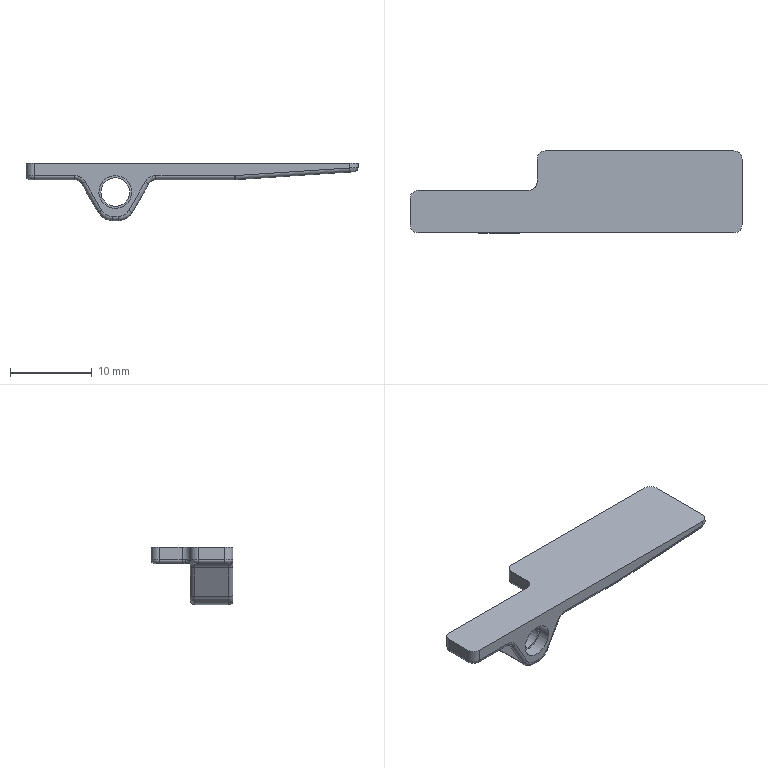NC program | Mastercam | posted with a generic post | part box 40.5 x 10 x 7 mm
Lines 3535 to 4637 of 12178:
(2 BM/BNOS |TOOL - 1|DIA. OFF. - 1|LEN. - 1|TOOL DIA. - 2.)
N7130 T1 M6
N7132 G0 G54 G90 X-19.75 Y.8 C0. B0. S8000 M3
N7134 G43 H1 Z25.
N7136 Z0.
N7138 G1 Z-5. F600.
N7140 Y4. F2000.
N7142 G0 Z0.
N7144 Z25.
N7146 X-19.67 Y4.258
N7148 Z0.
N7150 G1 Z-5. F600.
N7152 Y.538 F2000.
N7154 X-19.668 Y.512
N7156 X-19.662 Y.487
N7158 X-19.653 Y.463
N7160 X-19.642 Y.441
N7162 X-19.63 Y.424
N7164 X-19.619 Y.411
N7166 X-19.608 Y.405
N7168 X-19.599 Y.407
N7170 X-19.593 Y.417
N7172 X-19.591 Y.437
N7174 Y4.362
N7176 X-19.588 Y4.381
N7178 X-19.582 Y4.399
N7180 X-19.573 Y4.415
N7182 X-19.562 Y4.428
N7184 X-19.551 Y4.438
N7186 X-19.539 Y4.444
N7188 X-19.528 Y4.445
N7190 X-19.519 Y4.442
N7192 X-19.513 Y4.432
N7194 X-19.511 Y4.417
N7196 Y.382
N7198 X-19.509 Y.364
N7200 X-19.502 Y.348
N7202 X-19.494 Y.333
N7204 X-19.483 Y.322
N7206 X-19.471 Y.313
N7208 X-19.459 Y.308
N7210 X-19.448 Y.307
N7212 X-19.439 Y.311
N7214 X-19.433 Y.321
N7216 X-19.431 Y.336
N7218 Y4.465
N7220 X-19.429 Y4.481
N7222 X-19.423 Y4.493
N7224 X-19.414 Y4.503
N7226 X-19.403 Y4.51
N7228 X-19.391 Y4.514
N7230 X-19.379
N7232 X-19.369 Y4.511
N7234 X-19.36 Y4.505
N7236 X-19.354 Y4.495
N7238 X-19.351 Y4.481
N7240 Y.318
N7242 X-19.349 Y.303
N7244 X-19.343 Y.29
N7246 X-19.334 Y.28
N7248 X-19.323 Y.273
N7250 X-19.311 Y.268
N7252 X-19.3 Y.267
N7254 X-19.289 Y.27
N7256 X-19.28 Y.276
N7258 X-19.274 Y.286
N7260 X-19.272 Y.3
N7262 Y4.496
N7264 X-19.269 Y4.51
N7266 X-19.263 Y4.522
N7268 X-19.254 Y4.53
N7270 X-19.243 Y4.536
N7272 X-19.232 Y4.538
N7274 X-19.22 Y4.537
N7276 X-19.209 Y4.533
N7278 X-19.2 Y4.525
N7280 X-19.194 Y4.514
N7282 X-19.192 Y4.5
N7284 Y.3
N7286 X-19.19 Y.286
N7288 X-19.183 Y.274
N7290 X-19.175 Y.267
N7292 X-19.164 Y.262
N7294 X-19.152 Y.26
N7296 X-19.14 Y.262
N7298 X-19.129 Y.267
N7300 X-19.12 Y.274
N7302 X-19.114 Y.286
N7304 X-19.112 Y.3
N7306 Y4.5
N7308 X-19.11 Y4.514
N7310 X-19.104 Y4.526
N7312 X-19.095 Y4.533
N7314 X-19.084 Y4.538
N7316 X-19.072 Y4.54
N7318 X-19.06 Y4.538
N7320 X-19.05 Y4.533
N7322 X-19.041 Y4.526
N7324 X-19.035 Y4.514
N7326 X-19.032 Y4.5
N7328 Y.3
N7330 X-19.03 Y.286
N7332 X-19.024 Y.274
N7334 X-19.015 Y.267
N7336 X-19.004 Y.262
N7338 X-18.992 Y.26
N7340 X-18.981 Y.262
N7342 X-18.97 Y.267
N7344 X-18.961 Y.274
N7346 X-18.955 Y.286
N7348 X-18.953 Y.3
N7350 Y4.5
N7352 X-18.95 Y4.514
N7354 X-18.944 Y4.526
N7356 X-18.935 Y4.533
N7358 X-18.924 Y4.538
N7360 X-18.913 Y4.54
N7362 X-18.901 Y4.538
N7364 X-18.89 Y4.533
N7366 X-18.881 Y4.526
N7368 X-18.875 Y4.514
N7370 X-18.873 Y4.5
N7372 Y.3
N7374 X-18.871 Y.286
N7376 X-18.865 Y.274
N7378 X-18.856 Y.267
N7380 X-18.845 Y.262
N7382 X-18.833 Y.26
N7384 X-18.821 Y.262
N7386 X-18.81 Y.267
N7388 X-18.801 Y.274
N7390 X-18.795 Y.286
N7392 X-18.793 Y.3
N7394 Y4.5
N7396 X-18.791 Y4.514
N7398 X-18.785 Y4.526
N7400 X-18.776 Y4.533
N7402 X-18.765 Y4.538
N7404 X-18.753 Y4.54
N7406 X-18.741 Y4.538
N7408 X-18.731 Y4.533
N7410 X-18.722 Y4.526
N7412 X-18.716 Y4.514
N7414 X-18.713 Y4.5
N7416 Y.3
N7418 X-18.711 Y.286
N7420 X-18.705 Y.274
N7422 X-18.696 Y.267
N7424 X-18.685 Y.262
N7426 X-18.673 Y.26
N7428 X-18.662 Y.262
N7430 X-18.651 Y.267
N7432 X-18.642 Y.274
N7434 X-18.636 Y.286
N7436 X-18.634 Y.3
N7438 Y4.5
N7440 X-18.631 Y4.514
N7442 X-18.625 Y4.526
N7444 X-18.616 Y4.533
N7446 X-18.606 Y4.538
N7448 X-18.594 Y4.54
N7450 X-18.582 Y4.538
N7452 X-18.571 Y4.533
N7454 X-18.562 Y4.526
N7456 X-18.556 Y4.514
N7458 X-18.554 Y4.5
N7460 Y.3
N7462 X-18.552 Y.286
N7464 X-18.546 Y.274
N7466 X-18.537 Y.267
N7468 X-18.526 Y.262
N7470 X-18.514 Y.26
N7472 X-18.502 Y.262
N7474 X-18.491 Y.267
N7476 X-18.482 Y.274
N7478 X-18.476 Y.286
N7480 X-18.474 Y.3
N7482 Y4.5
N7484 X-18.472 Y4.514
N7486 X-18.466 Y4.526
N7488 X-18.457 Y4.533
N7490 X-18.446 Y4.538
N7492 X-18.434 Y4.54
N7494 X-18.422 Y4.538
N7496 X-18.412 Y4.533
N7498 X-18.403 Y4.526
N7500 X-18.397 Y4.514
N7502 X-18.394 Y4.5
N7504 Y.3
N7506 X-18.392 Y.286
N7508 X-18.386 Y.274
N7510 X-18.377 Y.267
N7512 X-18.366 Y.262
N7514 X-18.354 Y.26
N7516 X-18.343 Y.262
N7518 X-18.332 Y.267
N7520 X-18.323 Y.274
N7522 X-18.317 Y.286
N7524 X-18.315 Y.3
N7526 Y4.5
N7528 X-18.312 Y4.514
N7530 X-18.306 Y4.526
N7532 X-18.297 Y4.533
N7534 X-18.287 Y4.538
N7536 X-18.275 Y4.54
N7538 X-18.263 Y4.538
N7540 X-18.252 Y4.533
N7542 X-18.243 Y4.526
N7544 X-18.237 Y4.514
N7546 X-18.235 Y4.5
N7548 Y.3
N7550 X-18.233 Y.286
N7552 X-18.227 Y.274
N7554 X-18.218 Y.267
N7556 X-18.207 Y.262
N7558 X-18.195 Y.26
N7560 X-18.183 Y.262
N7562 X-18.172 Y.267
N7564 X-18.163 Y.274
N7566 X-18.157 Y.286
N7568 X-18.155 Y.3
N7570 Y4.5
N7572 X-18.153 Y4.514
N7574 X-18.147 Y4.526
N7576 X-18.138 Y4.533
N7578 X-18.127 Y4.538
N7580 X-18.115 Y4.54
N7582 X-18.103 Y4.538
N7584 X-18.093 Y4.533
N7586 X-18.084 Y4.526
N7588 X-18.078 Y4.514
N7590 X-18.075 Y4.5
N7592 Y.3
N7594 X-18.073 Y.286
N7596 X-18.067 Y.274
N7598 X-18.058 Y.267
N7600 X-18.047 Y.262
N7602 X-18.035 Y.26
N7604 X-18.024 Y.262
N7606 X-18.013 Y.267
N7608 X-18.004 Y.274
N7610 X-17.998 Y.286
N7612 X-17.996 Y.3
N7614 Y4.5
N7616 X-17.993 Y4.514
N7618 X-17.987 Y4.526
N7620 X-17.978 Y4.533
N7622 X-17.968 Y4.538
N7624 X-17.956 Y4.54
N7626 X-17.944 Y4.538
N7628 X-17.933 Y4.533
N7630 X-17.924 Y4.526
N7632 X-17.918 Y4.514
N7634 X-17.916 Y4.5
N7636 Y.3
N7638 X-17.914 Y.286
N7640 X-17.908 Y.274
N7642 X-17.899 Y.267
N7644 X-17.888 Y.262
N7646 X-17.876 Y.26
N7648 X-17.864 Y.262
N7650 X-17.853 Y.267
N7652 X-17.844 Y.274
N7654 X-17.838 Y.286
N7656 X-17.836 Y.3
N7658 Y4.5
N7660 X-17.834 Y4.514
N7662 X-17.828 Y4.526
N7664 X-17.819 Y4.533
N7666 X-17.808 Y4.538
N7668 X-17.796 Y4.54
N7670 X-17.784 Y4.538
N7672 X-17.774 Y4.533
N7674 X-17.765 Y4.526
N7676 X-17.759 Y4.514
N7678 X-17.756 Y4.5
N7680 Y.3
N7682 X-17.754 Y.286
N7684 X-17.748 Y.274
N7686 X-17.739 Y.267
N7688 X-17.728 Y.262
N7690 X-17.717 Y.26
N7692 X-17.705 Y.262
N7694 X-17.694 Y.267
N7696 X-17.685 Y.274
N7698 X-17.679 Y.286
N7700 X-17.677 Y.3
N7702 Y4.5
N7704 X-17.674 Y4.514
N7706 X-17.668 Y4.526
N7708 X-17.659 Y4.533
N7710 X-17.649 Y4.538
N7712 X-17.637 Y4.54
N7714 X-17.625 Y4.538
N7716 X-17.614 Y4.533
N7718 X-17.605 Y4.526
N7720 X-17.599 Y4.514
N7722 X-17.597 Y4.5
N7724 Y.3
N7726 X-17.595 Y.286
N7728 X-17.589 Y.274
N7730 X-17.58 Y.267
N7732 X-17.569 Y.262
N7734 X-17.557 Y.26
N7736 X-17.545 Y.262
N7738 X-17.534 Y.267
N7740 X-17.525 Y.274
N7742 X-17.519 Y.286
N7744 X-17.517 Y.3
N7746 Y4.5
N7748 X-17.515 Y4.514
N7750 X-17.509 Y4.526
N7752 X-17.5 Y4.533
N7754 X-17.489 Y4.538
N7756 X-17.477 Y4.54
N7758 X-17.465 Y4.538
N7760 X-17.455 Y4.533
N7762 X-17.446 Y4.526
N7764 X-17.44 Y4.514
N7766 X-17.437 Y4.5
N7768 Y.3
N7770 X-17.435 Y.286
N7772 X-17.429 Y.274
N7774 X-17.42 Y.267
N7776 X-17.409 Y.262
N7778 X-17.398 Y.26
N7780 X-17.386 Y.262
N7782 X-17.375 Y.267
N7784 X-17.366 Y.274
N7786 X-17.36 Y.286
N7788 X-17.358 Y.3
N7790 Y4.5
N7792 X-17.355 Y4.514
N7794 X-17.349 Y4.526
N7796 X-17.34 Y4.533
N7798 X-17.33 Y4.538
N7800 X-17.318 Y4.54
N7802 X-17.306 Y4.538
N7804 X-17.295 Y4.533
N7806 X-17.286 Y4.526
N7808 X-17.28 Y4.514
N7810 X-17.278 Y4.5
N7812 Y.3
N7814 X-17.276 Y.286
N7816 X-17.27 Y.274
N7818 X-17.261 Y.267
N7820 X-17.25 Y.262
N7822 X-17.238 Y.26
N7824 X-17.226 Y.262
N7826 X-17.215 Y.267
N7828 X-17.206 Y.274
N7830 X-17.2 Y.286
N7832 X-17.198 Y.3
N7834 Y4.5
N7836 X-17.196 Y4.514
N7838 X-17.19 Y4.526
N7840 X-17.181 Y4.533
N7842 X-17.17 Y4.538
N7844 X-17.158 Y4.54
N7846 X-17.146 Y4.538
N7848 X-17.136 Y4.533
N7850 X-17.127 Y4.526
N7852 X-17.121 Y4.514
N7854 X-17.118 Y4.5
N7856 Y.3
N7858 X-17.116 Y.286
N7860 X-17.11 Y.274
N7862 X-17.101 Y.267
N7864 X-17.09 Y.262
N7866 X-17.079 Y.26
N7868 X-17.067 Y.262
N7870 X-17.056 Y.267
N7872 X-17.047 Y.274
N7874 X-17.041 Y.286
N7876 X-17.039 Y.3
N7878 Y4.5
N7880 X-17.036 Y4.514
N7882 X-17.03 Y4.526
N7884 X-17.021 Y4.533
N7886 X-17.011 Y4.538
N7888 X-16.999 Y4.54
N7890 X-16.987 Y4.538
N7892 X-16.976 Y4.533
N7894 X-16.967 Y4.526
N7896 X-16.961 Y4.514
N7898 X-16.959 Y4.5
N7900 Y.3
N7902 X-16.957 Y.286
N7904 X-16.951 Y.274
N7906 X-16.942 Y.267
N7908 X-16.931 Y.262
N7910 X-16.919 Y.26
N7912 X-16.907 Y.262
N7914 X-16.896 Y.267
N7916 X-16.887 Y.274
N7918 X-16.881 Y.286
N7920 X-16.879 Y.3
N7922 Y4.5
N7924 X-16.877 Y4.514
N7926 X-16.871 Y4.526
N7928 X-16.862 Y4.533
N7930 X-16.851 Y4.538
N7932 X-16.839 Y4.54
N7934 X-16.828 Y4.538
N7936 X-16.817 Y4.533
N7938 X-16.808 Y4.526
N7940 X-16.802 Y4.514
N7942 X-16.799 Y4.5
N7944 Y.3
N7946 X-16.797 Y.286
N7948 X-16.791 Y.274
N7950 X-16.782 Y.267
N7952 X-16.771 Y.262
N7954 X-16.76 Y.26
N7956 X-16.748 Y.262
N7958 X-16.737 Y.267
N7960 X-16.728 Y.274
N7962 X-16.722 Y.286
N7964 X-16.72 Y.3
N7966 Y4.5
N7968 X-16.717 Y4.514
N7970 X-16.711 Y4.526
N7972 X-16.702 Y4.533
N7974 X-16.692 Y4.538
N7976 X-16.68 Y4.54
N7978 X-16.668 Y4.538
N7980 X-16.657 Y4.533
N7982 X-16.648 Y4.526
N7984 X-16.642 Y4.514
N7986 X-16.64 Y4.5
N7988 Y.3
N7990 X-16.638 Y.286
N7992 X-16.632 Y.274
N7994 X-16.623 Y.267
N7996 X-16.612 Y.262
N7998 X-16.6 Y.26
N8000 X-16.588 Y.262
N8002 X-16.577 Y.267
N8004 X-16.568 Y.274
N8006 X-16.562 Y.286
N8008 X-16.56 Y.3
N8010 Y4.5
N8012 X-16.558 Y4.514
N8014 X-16.552 Y4.526
N8016 X-16.543 Y4.533
N8018 X-16.532 Y4.538
N8020 X-16.52 Y4.54
N8022 X-16.509 Y4.538
N8024 X-16.498 Y4.533
N8026 X-16.489 Y4.526
N8028 X-16.483 Y4.514
N8030 X-16.48 Y4.5
N8032 Y.3
N8034 X-16.478 Y.286
N8036 X-16.472 Y.274
N8038 X-16.463 Y.267
N8040 X-16.452 Y.262
N8042 X-16.441 Y.26
N8044 X-16.429 Y.262
N8046 X-16.418 Y.267
N8048 X-16.409 Y.274
N8050 X-16.403 Y.286
N8052 X-16.401 Y.3
N8054 Y4.5
N8056 X-16.398 Y4.514
N8058 X-16.392 Y4.526
N8060 X-16.383 Y4.533
N8062 X-16.373 Y4.538
N8064 X-16.361 Y4.54
N8066 X-16.349 Y4.538
N8068 X-16.338 Y4.533
N8070 X-16.329 Y4.526
N8072 X-16.323 Y4.514
N8074 X-16.321 Y4.5
N8076 Y.3
N8078 X-16.319 Y.286
N8080 X-16.313 Y.274
N8082 X-16.304 Y.267
N8084 X-16.293 Y.262
N8086 X-16.281 Y.26
N8088 X-16.269 Y.262
N8090 X-16.258 Y.267
N8092 X-16.25 Y.274
N8094 X-16.243 Y.286
N8096 X-16.241 Y.3
N8098 Y4.5
N8100 X-16.239 Y4.514
N8102 X-16.233 Y4.526
N8104 X-16.224 Y4.533
N8106 X-16.213 Y4.538
N8108 X-16.201 Y4.54
N8110 X-16.19 Y4.538
N8112 X-16.179 Y4.533
N8114 X-16.17 Y4.526
N8116 X-16.164 Y4.514
N8118 X-16.161 Y4.5
N8120 Y.3
N8122 X-16.159 Y.286
N8124 X-16.153 Y.274
N8126 X-16.144 Y.267
N8128 X-16.133 Y.262
N8130 X-16.122 Y.26
N8132 X-16.11 Y.262
N8134 X-16.099 Y.267
N8136 X-16.09 Y.274
N8138 X-16.084 Y.286
N8140 X-16.082 Y.3
N8142 Y4.5
N8144 X-16.08 Y4.514
N8146 X-16.073 Y4.526
N8148 X-16.065 Y4.533
N8150 X-16.054 Y4.538
N8152 X-16.042 Y4.54
N8154 X-16.03 Y4.538
N8156 X-16.019 Y4.533
N8158 X-16.01 Y4.526
N8160 X-16.004 Y4.514
N8162 X-16.002 Y4.5
N8164 Y.3
N8166 X-16. Y.286
N8168 X-15.994 Y.274
N8170 X-15.985 Y.267
N8172 X-15.974 Y.262
N8174 X-15.962 Y.26
N8176 X-15.95 Y.262
N8178 X-15.939 Y.267
N8180 X-15.931 Y.274
N8182 X-15.924 Y.286
N8184 X-15.922 Y.3
N8186 Y4.5
N8188 X-15.92 Y4.514
N8190 X-15.914 Y4.526
N8192 X-15.905 Y4.533
N8194 X-15.894 Y4.538
N8196 X-15.882 Y4.54
N8198 X-15.871 Y4.538
N8200 X-15.86 Y4.533
N8202 X-15.851 Y4.526
N8204 X-15.845 Y4.514
N8206 X-15.843 Y4.5
N8208 Y.3
N8210 X-15.84 Y.286
N8212 X-15.834 Y.274
N8214 X-15.825 Y.267
N8216 X-15.814 Y.262
N8218 X-15.803 Y.26
N8220 X-15.791 Y.262
N8222 X-15.78 Y.267
N8224 X-15.771 Y.274
N8226 X-15.765 Y.286
N8228 X-15.763 Y.3
N8230 Y4.5
N8232 X-15.761 Y4.514
N8234 X-15.754 Y4.526
N8236 X-15.746 Y4.533
N8238 X-15.735 Y4.538
N8240 X-15.723 Y4.54
N8242 X-15.711 Y4.538
N8244 X-15.7 Y4.533
N8246 X-15.691 Y4.526
N8248 X-15.685 Y4.514
N8250 X-15.683 Y4.5
N8252 Y.3
N8254 X-15.681 Y.286
N8256 X-15.675 Y.274
N8258 X-15.666 Y.267
N8260 X-15.655 Y.262
N8262 X-15.643 Y.26
N8264 X-15.631 Y.262
N8266 X-15.62 Y.267
N8268 X-15.612 Y.274
N8270 X-15.606 Y.286
N8272 X-15.603 Y.3
N8274 Y4.5
N8276 X-15.601 Y4.514
N8278 X-15.595 Y4.526
N8280 X-15.586 Y4.533
N8282 X-15.575 Y4.538
N8284 X-15.563 Y4.54
N8286 X-15.552 Y4.538
N8288 X-15.541 Y4.533
N8290 X-15.532 Y4.526
N8292 X-15.526 Y4.514
N8294 X-15.524 Y4.5
N8296 Y.3
N8298 X-15.521 Y.286
N8300 X-15.515 Y.274
N8302 X-15.506 Y.267
N8304 X-15.495 Y.262
N8306 X-15.484 Y.26
N8308 X-15.472 Y.262
N8310 X-15.461 Y.267
N8312 X-15.452 Y.274
N8314 X-15.446 Y.286
N8316 X-15.444 Y.3
N8318 Y4.5
N8320 X-15.442 Y4.514
N8322 X-15.435 Y4.526
N8324 X-15.427 Y4.533
N8326 X-15.416 Y4.538
N8328 X-15.404 Y4.54
N8330 X-15.392 Y4.538
N8332 X-15.381 Y4.533
N8334 X-15.372 Y4.526
N8336 X-15.366 Y4.514
N8338 X-15.364 Y4.5
N8340 Y.3
N8342 X-15.362 Y.286
N8344 X-15.356 Y.274
N8346 X-15.347 Y.267
N8348 X-15.336 Y.262
N8350 X-15.324 Y.26
N8352 X-15.312 Y.262
N8354 X-15.302 Y.267
N8356 X-15.293 Y.274
N8358 X-15.287 Y.286
N8360 X-15.284 Y.3
N8362 Y4.5
N8364 X-15.282 Y4.514
N8366 X-15.276 Y4.526
N8368 X-15.267 Y4.533
N8370 X-15.256 Y4.538
N8372 X-15.244 Y4.54
N8374 X-15.233 Y4.538
N8376 X-15.222 Y4.533
N8378 X-15.213 Y4.526
N8380 X-15.207 Y4.514
N8382 X-15.205 Y4.5
N8384 Y.3
N8386 X-15.202 Y.286
N8388 X-15.196 Y.274
N8390 X-15.187 Y.267
N8392 X-15.176 Y.262
N8394 X-15.165 Y.26
N8396 X-15.153 Y.262
N8398 X-15.142 Y.267
N8400 X-15.133 Y.274
N8402 X-15.127 Y.286
N8404 X-15.125 Y.3
N8406 Y4.5
N8408 X-15.123 Y4.514
N8410 X-15.117 Y4.526
N8412 X-15.108 Y4.533
N8414 X-15.097 Y4.538
N8416 X-15.085 Y4.54
N8418 X-15.073 Y4.538
N8420 X-15.062 Y4.533
N8422 X-15.053 Y4.526
N8424 X-15.047 Y4.514
N8426 X-15.045 Y4.5
N8428 Y.3
N8430 X-15.043 Y.286
N8432 X-15.037 Y.274
N8434 X-15.028 Y.267
N8436 X-15.017 Y.262
N8438 X-15.005 Y.26
N8440 X-14.993 Y.262
N8442 X-14.983 Y.267
N8444 X-14.974 Y.274
N8446 X-14.968 Y.286
N8448 X-14.965 Y.3
N8450 Y4.5
N8452 X-14.963 Y4.514
N8454 X-14.957 Y4.526
N8456 X-14.948 Y4.533
N8458 X-14.937 Y4.538
N8460 X-14.925 Y4.54
N8462 X-14.914 Y4.538
N8464 X-14.903 Y4.533
N8466 X-14.894 Y4.526
N8468 X-14.888 Y4.514
N8470 X-14.886 Y4.5
N8472 Y.3
N8474 X-14.883 Y.286
N8476 X-14.877 Y.274
N8478 X-14.868 Y.267
N8480 X-14.857 Y.262
N8482 X-14.846 Y.26
N8484 X-14.834 Y.262
N8486 X-14.823 Y.267
N8488 X-14.814 Y.274
N8490 X-14.808 Y.286
N8492 X-14.806 Y.3
N8494 Y4.5
N8496 X-14.804 Y4.514
N8498 X-14.798 Y4.526
N8500 X-14.789 Y4.533
N8502 X-14.778 Y4.538
N8504 X-14.766 Y4.54
N8506 X-14.754 Y4.538
N8508 X-14.743 Y4.533
N8510 X-14.734 Y4.526
N8512 X-14.728 Y4.514
N8514 X-14.726 Y4.5
N8516 Y.3
N8518 X-14.724 Y.286
N8520 X-14.718 Y.274
N8522 X-14.709 Y.267
N8524 X-14.698 Y.262
N8526 X-14.686 Y.26
N8528 X-14.674 Y.262
N8530 X-14.664 Y.267
N8532 X-14.655 Y.274
N8534 X-14.649 Y.286
N8536 X-14.646 Y.3
N8538 Y4.5
N8540 X-14.644 Y4.514
N8542 X-14.638 Y4.526
N8544 X-14.629 Y4.533
N8546 X-14.618 Y4.538
N8548 X-14.606 Y4.54
N8550 X-14.595 Y4.538
N8552 X-14.584 Y4.533
N8554 X-14.575 Y4.526
N8556 X-14.569 Y4.514
N8558 X-14.567 Y4.5
N8560 Y.3
N8562 X-14.564 Y.286
N8564 X-14.558 Y.274
N8566 X-14.549 Y.267
N8568 X-14.539 Y.262
N8570 X-14.527 Y.26
N8572 X-14.515 Y.262
N8574 X-14.504 Y.267
N8576 X-14.495 Y.274
N8578 X-14.489 Y.286
N8580 X-14.487 Y.3
N8582 Y4.5
N8584 X-14.485 Y4.514
N8586 X-14.479 Y4.526
N8588 X-14.47 Y4.533
N8590 X-14.459 Y4.538
N8592 X-14.447 Y4.54
N8594 X-14.435 Y4.538
N8596 X-14.424 Y4.533
N8598 X-14.415 Y4.526
N8600 X-14.409 Y4.514
N8602 X-14.407 Y4.5
N8604 Y.3
N8606 X-14.405 Y.286
N8608 X-14.399 Y.274
N8610 X-14.39 Y.267
N8612 X-14.379 Y.262
N8614 X-14.367 Y.26
N8616 X-14.355 Y.262
N8618 X-14.345 Y.267
N8620 X-14.342 Y.269
N8622 X-14.338 Y.273 Z-4.999
N8624 X-14.336 Y.274 Z-4.998
N8626 X-14.33 Y.286 Z-4.996
N8628 X-14.327 Y.3 Z-4.991
N8630 Z-5.
N8632 Y4.5
N8634 Z-4.991
N8636 Z-4.993
N8638 Z-5.
N8640 Y.3
N8642 Z-4.991
N8644 Z-5.
N8646 Y4.5
N8648 Z-4.991
N8650 Z-5.
N8652 Y.3
N8654 Z-4.991
N8656 Z-5.
N8658 Y4.5
N8660 Z-4.991
N8662 Z-5.
N8664 Y.3
N8666 Z-4.991
N8668 Z-5.
N8670 Y4.5
N8672 Z-4.991
N8674 Z-5.
N8676 Y.3
N8678 Z-4.991
N8680 Z-5.
N8682 Y4.5
N8684 Z-4.991
N8686 Z-5.
N8688 Y.3
N8690 Z-4.991
N8692 Z-5.
N8694 Y4.5
N8696 Z-4.991
N8698 Z-5.
N8700 Y.3
N8702 Z-4.991
N8704 Z-5.
N8706 Y4.5
N8708 Z-4.991
N8710 Z-5.
N8712 Y.3
N8714 Y4.5
N8716 Z-4.991
N8718 Z-5.
N8720 Y.3
N8722 Z-4.991
N8724 Z-5.
N8726 Y4.5
N8728 Z-4.991
N8730 Z-5.
N8732 Y.3
N8734 Z-4.991
N8736 Z-5.
N8738 Y4.5
N8740 Z-4.991
N8742 X-14.326 Y4.514 Z-4.992
N8744 X-14.323 Y4.525 Z-4.99
N8746 X-14.32 Y4.531 Z-4.987
N8748 X-14.319 Y4.533 Z-4.985
N8750 X-14.314 Y4.537 Z-4.976
N8752 X-14.308 Y4.539 Z-4.966
N8754 X-14.302 Y4.537 Z-4.956
N8756 X-14.297 Y4.533 Z-4.947
N8758 X-14.293 Y4.525 Z-4.94
N8760 X-14.29 Y4.514 Z-4.935
N8762 X-14.288 Y4.5 Z-4.933
N8764 Y.3
N8766 X-14.287 Y.286 Z-4.931
N8768 X-14.284 Y.275 Z-4.926
N8770 X-14.28 Y.267 Z-4.918
N8772 X-14.275 Y.263 Z-4.909
N8774 X-14.269 Y.261 Z-4.899
N8776 X-14.263 Y.263 Z-4.889
N8778 X-14.258 Y.267 Z-4.88
N8780 X-14.254 Y.275 Z-4.872
N8782 X-14.251 Y.286 Z-4.867
N8784 X-14.25 Y.3 Z-4.865
N8786 Y4.5
N8788 X-14.249 Y4.514 Z-4.864
N8790 X-14.246 Y4.525 Z-4.858
N8792 X-14.241 Y4.533 Z-4.851
N8794 X-14.236 Y4.537 Z-4.842
N8796 X-14.23 Y4.539 Z-4.832
N8798 X-14.224 Y4.537 Z-4.822
N8800 X-14.219 Y4.533 Z-4.813
N8802 X-14.215 Y4.525 Z-4.805
N8804 X-14.212 Y4.514 Z-4.8
N8806 X-14.211 Y4.5 Z-4.798
N8808 Y.3
N8810 X-14.21 Y.286 Z-4.796
N8812 X-14.207 Y.275 Z-4.791
N8814 X-14.202 Y.267 Z-4.784
N8816 X-14.197 Y.263 Z-4.774
N8818 X-14.191 Y.261 Z-4.764
N8820 X-14.186 Y.263 Z-4.754
N8822 X-14.18 Y.267 Z-4.745
N8824 X-14.176 Y.275 Z-4.738
N8826 X-14.173 Y.286 Z-4.733
N8828 X-14.172 Y.3 Z-4.731
N8830 Y4.5
N8832 X-14.171 Y4.514 Z-4.729
N8834 X-14.168 Y4.525 Z-4.724
N8836 X-14.164 Y4.533 Z-4.716
N8838 X-14.158 Y4.537 Z-4.707
N8840 X-14.152 Y4.539 Z-4.697
N8842 X-14.147 Y4.537 Z-4.687
N8844 X-14.141 Y4.533 Z-4.678
N8846 X-14.137 Y4.525 Z-4.67
N8848 X-14.134 Y4.514 Z-4.665
N8850 X-14.133 Y4.5 Z-4.663
N8852 Y.3
N8854 X-14.132 Y.286 Z-4.662
N8856 X-14.129 Y.275 Z-4.656
N8858 X-14.125 Y.267 Z-4.649
N8860 X-14.119 Y.263 Z-4.64
N8862 X-14.114 Y.261 Z-4.63
N8864 X-14.108 Y.263 Z-4.62
N8866 X-14.103 Y.267 Z-4.611
N8868 X-14.098 Y.275 Z-4.603
N8870 X-14.095 Y.286 Z-4.598
N8872 X-14.094 Y.3 Z-4.596
N8874 Y4.5
N8876 X-14.093 Y4.514 Z-4.594
N8878 X-14.09 Y4.525 Z-4.589
N8880 X-14.086 Y4.533 Z-4.582
N8882 X-14.081 Y4.537 Z-4.572
N8884 X-14.075 Y4.539 Z-4.563
N8886 X-14.069 Y4.537 Z-4.553
N8888 X-14.064 Y4.533 Z-4.543
N8890 X-14.059 Y4.525 Z-4.536
N8892 X-14.056 Y4.514 Z-4.531
N8894 X-14.055 Y4.5 Z-4.529
N8896 Y.3
N8898 X-14.054 Y.286 Z-4.527
N8900 X-14.051 Y.275 Z-4.522
N8902 X-14.047 Y.267 Z-4.514
N8904 X-14.042 Y.263 Z-4.505
N8906 X-14.036 Y.261 Z-4.495
N8908 X-14.03 Y.263 Z-4.485
N8910 X-14.025 Y.267 Z-4.476
N8912 X-14.021 Y.275 Z-4.469
N8914 X-14.018 Y.286 Z-4.463
N8916 X-14.016 Y.3 Z-4.462
N8918 Y4.5
N8920 X-14.015 Y4.514 Z-4.46
N8922 X-14.012 Y4.525 Z-4.455
N8924 X-14.008 Y4.533 Z-4.447
N8926 X-14.003 Y4.537 Z-4.438
N8928 X-13.997 Y4.539 Z-4.428
N8930 X-13.991 Y4.537 Z-4.418
N8932 X-13.986 Y4.533 Z-4.409
N8934 X-13.982 Y4.525 Z-4.401
N8936 X-13.979 Y4.514 Z-4.396
N8938 X-13.978 Y4.5 Z-4.394
N8940 Y.3
N8942 X-13.977 Y.286 Z-4.392
N8944 X-13.974 Y.275 Z-4.387
N8946 X-13.969 Y.267 Z-4.38
N8948 X-13.964 Y.263 Z-4.371
N8950 X-13.958 Y.261 Z-4.361
N8952 X-13.952 Y.263 Z-4.351
N8954 X-13.947 Y.267 Z-4.341
N8956 X-13.943 Y.275 Z-4.334
N8958 X-13.94 Y.286 Z-4.329
N8960 X-13.939 Y.3 Z-4.327
N8962 Y4.5
N8964 X-13.938 Y4.514 Z-4.325
N8966 X-13.935 Y4.525 Z-4.32
N8968 X-13.93 Y4.533 Z-4.312
N8970 X-13.925 Y4.537 Z-4.303
N8972 X-13.919 Y4.539 Z-4.293
N8974 X-13.914 Y4.537 Z-4.283
N8976 X-13.908 Y4.533 Z-4.274
N8978 X-13.904 Y4.525 Z-4.267
N8980 X-13.901 Y4.514 Z-4.261
N8982 X-13.9 Y4.5 Z-4.26
N8984 Y.3
N8986 X-13.899 Y.286 Z-4.258
N8988 X-13.896 Y.275 Z-4.253
N8990 X-13.891 Y.267 Z-4.245
N8992 X-13.886 Y.263 Z-4.236
N8994 X-13.88 Y.261 Z-4.226
N8996 X-13.875 Y.263 Z-4.216
N8998 X-13.869 Y.267 Z-4.207
N9000 X-13.865 Y.275 Z-4.199
N9002 X-13.862 Y.286 Z-4.194
N9004 X-13.861 Y.3 Z-4.192
N9006 Y4.5
N9008 X-13.86 Y4.514 Z-4.19
N9010 X-13.857 Y4.525 Z-4.185
N9012 X-13.853 Y4.533 Z-4.178
N9014 X-13.847 Y4.537 Z-4.169
N9016 X-13.842 Y4.539 Z-4.159
N9018 X-13.836 Y4.537 Z-4.149
N9020 X-13.831 Y4.533 Z-4.14
N9022 X-13.826 Y4.525 Z-4.132
N9024 X-13.823 Y4.514 Z-4.127
N9026 X-13.822 Y4.5 Z-4.125
N9028 Y.3
N9030 X-13.821 Y.286 Z-4.123
N9032 X-13.818 Y.275 Z-4.118
N9034 X-13.814 Y.267 Z-4.11
N9036 X-13.808 Y.263 Z-4.101
N9038 X-13.803 Y.261 Z-4.091
N9040 X-13.797 Y.263 Z-4.081
N9042 X-13.792 Y.267 Z-4.072
N9044 X-13.787 Y.275 Z-4.065
N9046 X-13.784 Y.286 Z-4.06
N9048 X-13.783 Y.3 Z-4.058
N9050 Y4.5
N9052 X-13.782 Y4.514 Z-4.056
N9054 X-13.779 Y4.525 Z-4.051
N9056 X-13.775 Y4.533 Z-4.043
N9058 X-13.77 Y4.537 Z-4.034
N9060 X-13.764 Y4.539 Z-4.024
N9062 X-13.758 Y4.537 Z-4.014
N9064 X-13.753 Y4.533 Z-4.005
N9066 X-13.748 Y4.525 Z-3.997
N9068 X-13.746 Y4.514 Z-3.992
N9070 X-13.744 Y4.5 Z-3.99
N9072 Y.3
N9074 X-13.743 Y.286 Z-3.989
N9076 X-13.74 Y.275 Z-3.983
N9078 X-13.736 Y.267 Z-3.976
N9080 X-13.731 Y.263 Z-3.967
N9082 X-13.725 Y.261 Z-3.957
N9084 X-13.719 Y.263 Z-3.947
N9086 X-13.714 Y.267 Z-3.938
N9088 X-13.71 Y.275 Z-3.93
N9090 X-13.707 Y.286 Z-3.925
N9092 X-13.706 Y.3 Z-3.923
N9094 Y4.5
N9096 X-13.705 Y4.514 Z-3.921
N9098 X-13.702 Y4.525 Z-3.916
N9100 X-13.697 Y4.533 Z-3.909
N9102 X-13.692 Y4.537 Z-3.899
N9104 X-13.686 Y4.539 Z-3.889
N9106 X-13.68 Y4.537 Z-3.879
N9108 X-13.675 Y4.533 Z-3.87
N9110 X-13.671 Y4.525 Z-3.863
N9112 X-13.668 Y4.514 Z-3.858
N9114 X-13.667 Y4.5 Z-3.856
N9116 Y.3
N9118 X-13.666 Y.286 Z-3.854
N9120 X-13.663 Y.275 Z-3.849
N9122 X-13.658 Y.267 Z-3.841
N9124 X-13.653 Y.263 Z-3.832
N9126 X-13.647 Y.261 Z-3.822
N9128 X-13.642 Y.263 Z-3.812
N9130 X-13.636 Y.267 Z-3.803
N9132 X-13.632 Y.275 Z-3.795
N9134 X-13.629 Y.286 Z-3.79
N9136 X-13.628 Y.3 Z-3.788
N9138 Y4.5
N9140 X-13.627 Y4.514 Z-3.787
N9142 X-13.624 Y4.525 Z-3.781
N9144 X-13.619 Y4.533 Z-3.774
N9146 X-13.614 Y4.537 Z-3.765
N9148 X-13.608 Y4.539 Z-3.755
N9150 X-13.603 Y4.537 Z-3.745
N9152 X-13.597 Y4.533 Z-3.736
N9154 X-13.593 Y4.525 Z-3.728
N9156 X-13.59 Y4.514 Z-3.723
N9158 X-13.589 Y4.5 Z-3.721
N9160 Y.3
N9162 X-13.588 Y.286 Z-3.719
N9164 X-13.585 Y.275 Z-3.714
N9166 X-13.581 Y.267 Z-3.707
N9168 X-13.575 Y.263 Z-3.697
N9170 X-13.57 Y.261 Z-3.688
N9172 X-13.564 Y.263 Z-3.678
N9174 X-13.559 Y.267 Z-3.668
N9176 X-13.554 Y.275 Z-3.661
N9178 X-13.551 Y.286 Z-3.656
N9180 X-13.55 Y.3 Z-3.654
N9182 Y4.5
N9184 X-13.549 Y4.514 Z-3.652
N9186 X-13.546 Y4.525 Z-3.647
N9188 X-13.542 Y4.533 Z-3.639
N9190 X-13.536 Y4.537 Z-3.63
N9192 X-13.531 Y4.539 Z-3.62
N9194 X-13.525 Y4.537 Z-3.61
N9196 X-13.52 Y4.533 Z-3.601
N9198 X-13.515 Y4.525 Z-3.594
N9200 X-13.512 Y4.514 Z-3.588
N9202 X-13.511 Y4.5 Z-3.587
N9204 Y.3
N9206 X-13.51 Y.286 Z-3.585
N9208 X-13.507 Y.275 Z-3.58
N9210 X-13.503 Y.267 Z-3.572
N9212 X-13.498 Y.263 Z-3.563
N9214 X-13.492 Y.261 Z-3.553
N9216 X-13.486 Y.263 Z-3.543
N9218 X-13.481 Y.267 Z-3.534
N9220 X-13.476 Y.275 Z-3.526
N9222 X-13.474 Y.286 Z-3.521
N9224 X-13.472 Y.3 Z-3.519
N9226 Y4.5
N9228 X-13.471 Y4.514 Z-3.517
N9230 X-13.468 Y4.525 Z-3.512
N9232 X-13.464 Y4.533 Z-3.505
N9234 X-13.459 Y4.537 Z-3.496
N9236 X-13.453 Y4.539 Z-3.486
N9238 X-13.447 Y4.537 Z-3.476
N9240 X-13.442 Y4.533 Z-3.466
N9242 X-13.438 Y4.525 Z-3.459
N9244 X-13.435 Y4.514 Z-3.454
N9246 X-13.434 Y4.5 Z-3.452
N9248 Y.3
N9250 X-13.432 Y.286 Z-3.45
N9252 X-13.43 Y.275 Z-3.445
N9254 X-13.425 Y.267 Z-3.437
N9256 X-13.42 Y.263 Z-3.428
N9258 X-13.414 Y.261 Z-3.418
N9260 X-13.408 Y.263 Z-3.408
N9262 X-13.403 Y.267 Z-3.399
N9264 X-13.399 Y.275 Z-3.392
N9266 X-13.396 Y.286 Z-3.386
N9268 X-13.395 Y.3 Z-3.385
N9270 Y4.5
N9272 X-13.394 Y4.514 Z-3.383
N9274 X-13.391 Y4.525 Z-3.378
N9276 X-13.386 Y4.533 Z-3.37
N9278 X-13.381 Y4.537 Z-3.361
N9280 X-13.375 Y4.539 Z-3.351
N9282 X-13.37 Y4.537 Z-3.341
N9284 X-13.364 Y4.533 Z-3.332
N9286 X-13.36 Y4.525 Z-3.324
N9288 X-13.357 Y4.514 Z-3.319
N9290 X-13.356 Y4.5 Z-3.317
N9292 Y.3
N9294 X-13.355 Y.286 Z-3.315
N9296 X-13.352 Y.275 Z-3.31
N9298 X-13.347 Y.267 Z-3.303
N9300 X-13.342 Y.263 Z-3.294
N9302 X-13.336 Y.261 Z-3.284
N9304 X-13.331 Y.263 Z-3.274
N9306 X-13.325 Y.267 Z-3.265
N9308 X-13.321 Y.275 Z-3.257
N9310 X-13.318 Y.286 Z-3.252
N9312 X-13.317 Y.3 Z-3.25
N9314 Y4.5
N9316 X-13.316 Y4.514 Z-3.248
N9318 X-13.313 Y4.525 Z-3.243
N9320 X-13.309 Y4.533 Z-3.235
N9322 X-13.303 Y4.537 Z-3.226
N9324 X-13.298 Y4.539 Z-3.216
N9326 X-13.292 Y4.537 Z-3.206
N9328 X-13.287 Y4.533 Z-3.197
N9330 X-13.282 Y4.525 Z-3.19
N9332 X-13.279 Y4.514 Z-3.185